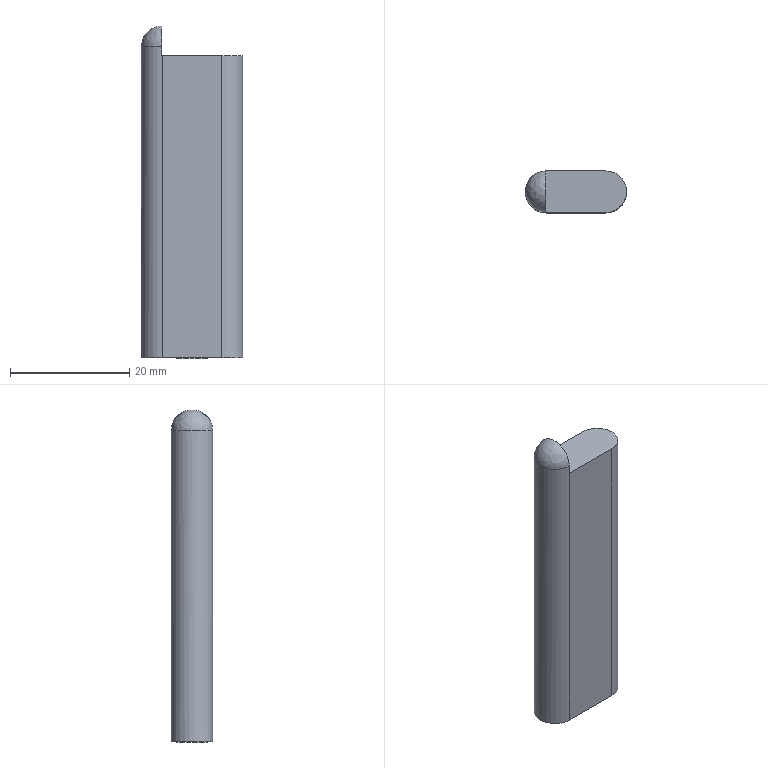Part | STEP file | LUOI GA TRON TREN | 1 solid | 15 faces | box 17 x 7 x 55.799 mm | volume 5306 mm3 | cylinder 5 | plane 5 | cone 4 | spline 1 | commonest cylinder face diameters 7 x3 4.134 x2
STEP:
#1=CARTESIAN_POINT('',(0.,0.,0.));
#2=DIRECTION('',(0.,0.,1.));
#3=DIRECTION('',(1.,0.,0.));
#4=AXIS2_PLACEMENT_3D('',#1,#2,#3);
#5=CARTESIAN_POINT('',(-3.5,0.,0.));
#6=VERTEX_POINT('',#5);
#7=CARTESIAN_POINT('',(0.,3.5,0.));
#8=VERTEX_POINT('',#7);
#9=CARTESIAN_POINT('',(-3.5,3.5,0.));
#10=DIRECTION('',(0.,0.,1.));
#11=DIRECTION('',(1.,0.,0.));
#12=AXIS2_PLACEMENT_3D('',#9,#10,#11);
#13=CIRCLE('',#12,3.5);
#14=CARTESIAN_POINT('',(-3.5,3.5,0.));
#15=DIRECTION('',(0.,0.,1.));
#16=DIRECTION('',(1.,0.,0.));
#17=AXIS2_PLACEMENT_3D('',#14,#15,#16);
#18=CYLINDRICAL_SURFACE('',#17,3.5);
#19=CARTESIAN_POINT('',(0.,0.));
#20=DIRECTION('',(1.,0.));
#21=VECTOR('',#20,1.);
#22=LINE('',#19,#21);
#23=(GEOMETRIC_REPRESENTATION_CONTEXT(2)PARAMETRIC_REPRESENTATION_CONTEXT()REPRESENTATION_CONTEXT('',''));
#24=DEFINITIONAL_REPRESENTATION('',(#22),#23);
#25=PCURVE('',#18,#24);
#26=CARTESIAN_POINT('',(-8.5,3.5,0.));
#27=DIRECTION('',(0.,0.,1.));
#28=DIRECTION('',(1.,0.,0.));
#29=AXIS2_PLACEMENT_3D('',#26,#27,#28);
#30=PLANE('',#29);
#31=CARTESIAN_POINT('',(5.,0.));
#32=DIRECTION('',(1.,0.));
#33=AXIS2_PLACEMENT_2D('',#31,#32);
#34=CIRCLE('',#33,3.5);
#35=(GEOMETRIC_REPRESENTATION_CONTEXT(2)PARAMETRIC_REPRESENTATION_CONTEXT()REPRESENTATION_CONTEXT('',''));
#36=DEFINITIONAL_REPRESENTATION('',(#34),#35);
#37=PCURVE('',#30,#36);
#38=SURFACE_CURVE('',#13,(#25,#37),.PCURVE_S1.);
#39=EDGE_CURVE('',#6,#8,#38,.T.);
#40=ORIENTED_EDGE('',*,*,#39,.T.);
#41=CARTESIAN_POINT('',(0.,3.5,50.8));
#42=VERTEX_POINT('',#41);
#43=CARTESIAN_POINT('',(0.,3.5,0.));
#44=DIRECTION('',(0.,0.,1.));
#45=VECTOR('',#44,1.);
#46=LINE('',#43,#45);
#47=CARTESIAN_POINT('',(6.283,0.));
#48=DIRECTION('',(0.,1.));
#49=VECTOR('',#48,1.);
#50=LINE('',#47,#49);
#51=(GEOMETRIC_REPRESENTATION_CONTEXT(2)PARAMETRIC_REPRESENTATION_CONTEXT()REPRESENTATION_CONTEXT('',''));
#52=DEFINITIONAL_REPRESENTATION('',(#50),#51);
#53=PCURVE('',#18,#52);
#54=CARTESIAN_POINT('',(-3.5,3.5,0.));
#55=DIRECTION('',(0.,0.,1.));
#56=DIRECTION('',(1.,0.,0.));
#57=AXIS2_PLACEMENT_3D('',#54,#55,#56);
#58=CYLINDRICAL_SURFACE('',#57,3.5);
#59=CARTESIAN_POINT('',(0.,0.));
#60=DIRECTION('',(0.,1.));
#61=VECTOR('',#60,1.);
#62=LINE('',#59,#61);
#63=(GEOMETRIC_REPRESENTATION_CONTEXT(2)PARAMETRIC_REPRESENTATION_CONTEXT()REPRESENTATION_CONTEXT('',''));
#64=DEFINITIONAL_REPRESENTATION('',(#62),#63);
#65=PCURVE('',#58,#64);
#66=SURFACE_CURVE('',#46,(#53,#65),.PCURVE_S1.);
#67=EDGE_CURVE('',#8,#42,#66,.T.);
#68=ORIENTED_EDGE('',*,*,#67,.T.);
#69=CARTESIAN_POINT('',(-3.5,0.,50.8));
#70=VERTEX_POINT('',#69);
#71=CARTESIAN_POINT('',(-3.5,3.5,50.8));
#72=DIRECTION('',(0.,0.,-1.));
#73=DIRECTION('',(1.,0.,0.));
#74=AXIS2_PLACEMENT_3D('',#71,#72,#73);
#75=CIRCLE('',#74,3.5);
#76=CARTESIAN_POINT('',(6.283,50.8));
#77=DIRECTION('',(-1.,0.));
#78=VECTOR('',#77,1.);
#79=LINE('',#76,#78);
#80=(GEOMETRIC_REPRESENTATION_CONTEXT(2)PARAMETRIC_REPRESENTATION_CONTEXT()REPRESENTATION_CONTEXT('',''));
#81=DEFINITIONAL_REPRESENTATION('',(#79),#80);
#82=PCURVE('',#18,#81);
#83=CARTESIAN_POINT('',(-13.6,0.,50.8));
#84=DIRECTION('',(0.,0.,-1.));
#85=DIRECTION('',(-1.,0.,0.));
#86=AXIS2_PLACEMENT_3D('',#83,#84,#85);
#87=PLANE('',#86);
#88=CARTESIAN_POINT('',(-10.1,3.5));
#89=DIRECTION('',(-1.,0.));
#90=AXIS2_PLACEMENT_2D('',#88,#89);
#91=CIRCLE('',#90,3.5);
#92=(GEOMETRIC_REPRESENTATION_CONTEXT(2)PARAMETRIC_REPRESENTATION_CONTEXT()REPRESENTATION_CONTEXT('',''));
#93=DEFINITIONAL_REPRESENTATION('',(#91),#92);
#94=PCURVE('',#87,#93);
#95=SURFACE_CURVE('',#75,(#82,#94),.PCURVE_S1.);
#96=EDGE_CURVE('',#42,#70,#95,.T.);
#97=ORIENTED_EDGE('',*,*,#96,.T.);
#98=CARTESIAN_POINT('',(-3.5,0.,0.));
#99=DIRECTION('',(0.,0.,1.));
#100=VECTOR('',#99,1.);
#101=LINE('',#98,#100);
#102=CARTESIAN_POINT('',(4.712,0.));
#103=DIRECTION('',(0.,1.));
#104=VECTOR('',#103,1.);
#105=LINE('',#102,#104);
#106=(GEOMETRIC_REPRESENTATION_CONTEXT(2)PARAMETRIC_REPRESENTATION_CONTEXT()REPRESENTATION_CONTEXT('',''));
#107=DEFINITIONAL_REPRESENTATION('',(#105),#106);
#108=PCURVE('',#18,#107);
#109=CARTESIAN_POINT('',(0.,0.,0.));
#110=DIRECTION('',(0.,-1.,0.));
#111=DIRECTION('',(0.,0.,-1.));
#112=AXIS2_PLACEMENT_3D('',#109,#110,#111);
#113=PLANE('',#112);
#114=CARTESIAN_POINT('',(0.,-3.5));
#115=DIRECTION('',(-1.,0.));
#116=VECTOR('',#115,1.);
#117=LINE('',#114,#116);
#118=(GEOMETRIC_REPRESENTATION_CONTEXT(2)PARAMETRIC_REPRESENTATION_CONTEXT()REPRESENTATION_CONTEXT('',''));
#119=DEFINITIONAL_REPRESENTATION('',(#117),#118);
#120=PCURVE('',#113,#119);
#121=SURFACE_CURVE('',#101,(#108,#120),.PCURVE_S1.);
#122=EDGE_CURVE('',#6,#70,#121,.T.);
#123=ORIENTED_EDGE('',*,*,#122,.F.);
#124=EDGE_LOOP('',(#40,#68,#97,#123));
#125=FACE_BOUND('',#124,.T.);
#126=ADVANCED_FACE('',(#125),#18,.T.);
#127=CARTESIAN_POINT('',(-10.567,3.5,0.5));
#128=VERTEX_POINT('',#127);
#129=CARTESIAN_POINT('',(-11.067,3.5,0.));
#130=VERTEX_POINT('',#129);
#131=CARTESIAN_POINT('',(-11.067,3.5,0.));
#132=DIRECTION('',(-0.7071,0.,-0.7071));
#133=VECTOR('',#132,1.);
#134=LINE('',#131,#133);
#135=CARTESIAN_POINT('',(-8.5,3.5,0.));
#136=DIRECTION('',(0.,0.,-1.));
#137=DIRECTION('',(-1.,0.,0.));
#138=AXIS2_PLACEMENT_3D('',#135,#136,#137);
#139=CONICAL_SURFACE('',#138,2.567,0.7854);
#140=CARTESIAN_POINT('',(6.283,0.));
#141=DIRECTION('',(0.,1.));
#142=VECTOR('',#141,1.);
#143=LINE('',#140,#142);
#144=(GEOMETRIC_REPRESENTATION_CONTEXT(2)PARAMETRIC_REPRESENTATION_CONTEXT()REPRESENTATION_CONTEXT('',''));
#145=DEFINITIONAL_REPRESENTATION('',(#143),#144);
#146=PCURVE('',#139,#145);
#147=CARTESIAN_POINT('',(-8.5,3.5,0.));
#148=DIRECTION('',(0.,0.,-1.));
#149=DIRECTION('',(-1.,0.,0.));
#150=AXIS2_PLACEMENT_3D('',#147,#148,#149);
#151=CONICAL_SURFACE('',#150,2.567,0.7854);
#152=CARTESIAN_POINT('',(0.,0.));
#153=DIRECTION('',(0.,1.));
#154=VECTOR('',#153,1.);
#155=LINE('',#152,#154);
#156=(GEOMETRIC_REPRESENTATION_CONTEXT(2)PARAMETRIC_REPRESENTATION_CONTEXT()REPRESENTATION_CONTEXT('',''));
#157=DEFINITIONAL_REPRESENTATION('',(#155),#156);
#158=PCURVE('',#151,#157);
#159=SURFACE_CURVE('',#134,(#146,#158),.PCURVE_S1.);
#160=EDGE_CURVE('',#128,#130,#159,.T.);
#161=ORIENTED_EDGE('',*,*,#160,.T.);
#162=CARTESIAN_POINT('',(-5.933,3.5,0.));
#163=VERTEX_POINT('',#162);
#164=CARTESIAN_POINT('',(-8.5,3.5,0.));
#165=DIRECTION('',(0.,0.,-1.));
#166=DIRECTION('',(-1.,0.,0.));
#167=AXIS2_PLACEMENT_3D('',#164,#165,#166);
#168=CIRCLE('',#167,2.567);
#169=CARTESIAN_POINT('',(0.,0.));
#170=DIRECTION('',(1.,0.));
#171=VECTOR('',#170,1.);
#172=LINE('',#169,#171);
#173=(GEOMETRIC_REPRESENTATION_CONTEXT(2)PARAMETRIC_REPRESENTATION_CONTEXT()REPRESENTATION_CONTEXT('',''));
#174=DEFINITIONAL_REPRESENTATION('',(#172),#173);
#175=PCURVE('',#139,#174);
#176=CARTESIAN_POINT('',(-2.567,0.));
#177=CARTESIAN_POINT('',(-2.567,4.446));
#178=CARTESIAN_POINT('',(1.283,2.223));
#179=CARTESIAN_POINT('',(5.134,0.));
#180=CARTESIAN_POINT('',(1.283,-2.223));
#181=CARTESIAN_POINT('',(-2.567,-4.446));
#182=CARTESIAN_POINT('',(-2.567,0.));
#183=(BOUNDED_CURVE()B_SPLINE_CURVE(2,(#176,#177,#178,#179,#180,#181,#182),.UNSPECIFIED.,.T.,.F.)B_SPLINE_CURVE_WITH_KNOTS((1,2,2,2,2,1),(-2.094,0.,2.094,4.189,6.283,8.378),.UNSPECIFIED.)CURVE()GEOMETRIC_REPRESENTATION_ITEM()RATIONAL_B_SPLINE_CURVE((1.,0.5,1.,0.5,1.,0.5,1.))REPRESENTATION_ITEM(''));
#184=(GEOMETRIC_REPRESENTATION_CONTEXT(2)PARAMETRIC_REPRESENTATION_CONTEXT()REPRESENTATION_CONTEXT('',''));
#185=DEFINITIONAL_REPRESENTATION('',(#183),#184);
#186=PCURVE('',#30,#185);
#187=SURFACE_CURVE('',#168,(#175,#186),.PCURVE_S1.);
#188=EDGE_CURVE('',#163,#130,#187,.T.);
#189=ORIENTED_EDGE('',*,*,#188,.F.);
#190=CARTESIAN_POINT('',(-6.433,3.5,0.5));
#191=VERTEX_POINT('',#190);
#192=CARTESIAN_POINT('',(-5.933,3.5,0.));
#193=DIRECTION('',(0.7071,0.,-0.7071));
#194=VECTOR('',#193,1.);
#195=LINE('',#192,#194);
#196=CARTESIAN_POINT('',(3.142,0.));
#197=DIRECTION('',(0.,1.));
#198=VECTOR('',#197,1.);
#199=LINE('',#196,#198);
#200=(GEOMETRIC_REPRESENTATION_CONTEXT(2)PARAMETRIC_REPRESENTATION_CONTEXT()REPRESENTATION_CONTEXT('',''));
#201=DEFINITIONAL_REPRESENTATION('',(#199),#200);
#202=PCURVE('',#139,#201);
#203=CARTESIAN_POINT('',(3.142,0.));
#204=DIRECTION('',(0.,1.));
#205=VECTOR('',#204,1.);
#206=LINE('',#203,#205);
#207=(GEOMETRIC_REPRESENTATION_CONTEXT(2)PARAMETRIC_REPRESENTATION_CONTEXT()REPRESENTATION_CONTEXT('',''));
#208=DEFINITIONAL_REPRESENTATION('',(#206),#207);
#209=PCURVE('',#151,#208);
#210=SURFACE_CURVE('',#195,(#202,#209),.PCURVE_S1.);
#211=EDGE_CURVE('',#191,#163,#210,.T.);
#212=ORIENTED_EDGE('',*,*,#211,.F.);
#213=CARTESIAN_POINT('',(-8.5,3.5,0.5));
#214=DIRECTION('',(0.,0.,-1.));
#215=DIRECTION('',(1.,0.,0.));
#216=AXIS2_PLACEMENT_3D('',#213,#214,#215);
#217=CIRCLE('',#216,2.067);
#218=CARTESIAN_POINT('',(3.142,-0.5));
#219=DIRECTION('',(1.,0.));
#220=VECTOR('',#219,1.);
#221=LINE('',#218,#220);
#222=(GEOMETRIC_REPRESENTATION_CONTEXT(2)PARAMETRIC_REPRESENTATION_CONTEXT()REPRESENTATION_CONTEXT('',''));
#223=DEFINITIONAL_REPRESENTATION('',(#221),#222);
#224=PCURVE('',#139,#223);
#225=CARTESIAN_POINT('',(-8.5,3.5,10.));
#226=DIRECTION('',(0.,0.,-1.));
#227=DIRECTION('',(-1.,0.,0.));
#228=AXIS2_PLACEMENT_3D('',#225,#226,#227);
#229=CYLINDRICAL_SURFACE('',#228,2.067);
#230=CARTESIAN_POINT('',(3.142,9.5));
#231=DIRECTION('',(1.,0.));
#232=VECTOR('',#231,1.);
#233=LINE('',#230,#232);
#234=(GEOMETRIC_REPRESENTATION_CONTEXT(2)PARAMETRIC_REPRESENTATION_CONTEXT()REPRESENTATION_CONTEXT('',''));
#235=DEFINITIONAL_REPRESENTATION('',(#233),#234);
#236=PCURVE('',#229,#235);
#237=SURFACE_CURVE('',#217,(#224,#236),.PCURVE_S1.);
#238=EDGE_CURVE('',#191,#128,#237,.T.);
#239=ORIENTED_EDGE('',*,*,#238,.T.);
#240=EDGE_LOOP('',(#161,#189,#212,#239));
#241=FACE_BOUND('',#240,.F.);
#242=ADVANCED_FACE('',(#241),#139,.F.);
#243=CARTESIAN_POINT('',(-10.567,3.5,20.));
#244=VERTEX_POINT('',#243);
#245=CARTESIAN_POINT('',(-10.567,3.5,10.));
#246=DIRECTION('',(0.,0.,-1.));
#247=VECTOR('',#246,1.);
#248=LINE('',#245,#247);
#249=CARTESIAN_POINT('',(6.283,0.));
#250=DIRECTION('',(0.,1.));
#251=VECTOR('',#250,1.);
#252=LINE('',#249,#251);
#253=(GEOMETRIC_REPRESENTATION_CONTEXT(2)PARAMETRIC_REPRESENTATION_CONTEXT()REPRESENTATION_CONTEXT('',''));
#254=DEFINITIONAL_REPRESENTATION('',(#252),#253);
#255=PCURVE('',#229,#254);
#256=CARTESIAN_POINT('',(-8.5,3.5,10.));
#257=DIRECTION('',(0.,0.,-1.));
#258=DIRECTION('',(-1.,0.,0.));
#259=AXIS2_PLACEMENT_3D('',#256,#257,#258);
#260=CYLINDRICAL_SURFACE('',#259,2.067);
#261=CARTESIAN_POINT('',(0.,0.));
#262=DIRECTION('',(0.,1.));
#263=VECTOR('',#262,1.);
#264=LINE('',#261,#263);
#265=(GEOMETRIC_REPRESENTATION_CONTEXT(2)PARAMETRIC_REPRESENTATION_CONTEXT()REPRESENTATION_CONTEXT('',''));
#266=DEFINITIONAL_REPRESENTATION('',(#264),#265);
#267=PCURVE('',#260,#266);
#268=SURFACE_CURVE('',#248,(#255,#267),.PCURVE_S1.);
#269=EDGE_CURVE('',#244,#128,#268,.T.);
#270=ORIENTED_EDGE('',*,*,#269,.T.);
#271=ORIENTED_EDGE('',*,*,#238,.F.);
#272=CARTESIAN_POINT('',(-6.433,3.5,20.));
#273=VERTEX_POINT('',#272);
#274=CARTESIAN_POINT('',(-6.433,3.5,10.));
#275=DIRECTION('',(0.,0.,-1.));
#276=VECTOR('',#275,1.);
#277=LINE('',#274,#276);
#278=CARTESIAN_POINT('',(3.142,0.));
#279=DIRECTION('',(0.,1.));
#280=VECTOR('',#279,1.);
#281=LINE('',#278,#280);
#282=(GEOMETRIC_REPRESENTATION_CONTEXT(2)PARAMETRIC_REPRESENTATION_CONTEXT()REPRESENTATION_CONTEXT('',''));
#283=DEFINITIONAL_REPRESENTATION('',(#281),#282);
#284=PCURVE('',#229,#283);
#285=CARTESIAN_POINT('',(3.142,0.));
#286=DIRECTION('',(0.,1.));
#287=VECTOR('',#286,1.);
#288=LINE('',#285,#287);
#289=(GEOMETRIC_REPRESENTATION_CONTEXT(2)PARAMETRIC_REPRESENTATION_CONTEXT()REPRESENTATION_CONTEXT('',''));
#290=DEFINITIONAL_REPRESENTATION('',(#288),#289);
#291=PCURVE('',#260,#290);
#292=SURFACE_CURVE('',#277,(#284,#291),.PCURVE_S1.);
#293=EDGE_CURVE('',#273,#191,#292,.T.);
#294=ORIENTED_EDGE('',*,*,#293,.F.);
#295=CARTESIAN_POINT('',(-8.5,3.5,20.));
#296=DIRECTION('',(0.,0.,-1.));
#297=DIRECTION('',(-1.,0.,0.));
#298=AXIS2_PLACEMENT_3D('',#295,#296,#297);
#299=CIRCLE('',#298,2.067);
#300=CARTESIAN_POINT('',(0.,-10.));
#301=DIRECTION('',(1.,0.));
#302=VECTOR('',#301,1.);
#303=LINE('',#300,#302);
#304=(GEOMETRIC_REPRESENTATION_CONTEXT(2)PARAMETRIC_REPRESENTATION_CONTEXT()REPRESENTATION_CONTEXT('',''));
#305=DEFINITIONAL_REPRESENTATION('',(#303),#304);
#306=PCURVE('',#229,#305);
#307=CARTESIAN_POINT('',(-8.5,3.5,20.));
#308=DIRECTION('',(0.,0.,-1.));
#309=DIRECTION('',(-1.,0.,0.));
#310=AXIS2_PLACEMENT_3D('',#307,#308,#309);
#311=CONICAL_SURFACE('',#310,2.067,1.03);
#312=CARTESIAN_POINT('',(0.,0.));
#313=DIRECTION('',(1.,0.));
#314=VECTOR('',#313,1.);
#315=LINE('',#312,#314);
#316=(GEOMETRIC_REPRESENTATION_CONTEXT(2)PARAMETRIC_REPRESENTATION_CONTEXT()REPRESENTATION_CONTEXT('',''));
#317=DEFINITIONAL_REPRESENTATION('',(#315),#316);
#318=PCURVE('',#311,#317);
#319=SURFACE_CURVE('',#299,(#306,#318),.PCURVE_S1.);
#320=EDGE_CURVE('',#273,#244,#319,.T.);
#321=ORIENTED_EDGE('',*,*,#320,.T.);
#322=EDGE_LOOP('',(#270,#271,#294,#321));
#323=FACE_BOUND('',#322,.F.);
#324=ADVANCED_FACE('',(#323),#229,.F.);
#325=ORIENTED_EDGE('',*,*,#320,.F.);
#326=CARTESIAN_POINT('',(-8.5,3.5,21.242));
#327=VERTEX_POINT('',#326);
#328=CARTESIAN_POINT('',(-6.433,3.5,20.));
#329=DIRECTION('',(0.8572,0.,-0.515));
#330=VECTOR('',#329,1.);
#331=LINE('',#328,#330);
#332=CARTESIAN_POINT('',(3.142,0.));
#333=DIRECTION('',(0.,1.));
#334=VECTOR('',#333,1.);
#335=LINE('',#332,#334);
#336=(GEOMETRIC_REPRESENTATION_CONTEXT(2)PARAMETRIC_REPRESENTATION_CONTEXT()REPRESENTATION_CONTEXT('',''));
#337=DEFINITIONAL_REPRESENTATION('',(#335),#336);
#338=PCURVE('',#311,#337);
#339=CARTESIAN_POINT('',(-8.5,3.5,20.));
#340=DIRECTION('',(0.,0.,-1.));
#341=DIRECTION('',(-1.,0.,0.));
#342=AXIS2_PLACEMENT_3D('',#339,#340,#341);
#343=CONICAL_SURFACE('',#342,2.067,1.03);
#344=CARTESIAN_POINT('',(3.142,0.));
#345=DIRECTION('',(0.,1.));
#346=VECTOR('',#345,1.);
#347=LINE('',#344,#346);
#348=(GEOMETRIC_REPRESENTATION_CONTEXT(2)PARAMETRIC_REPRESENTATION_CONTEXT()REPRESENTATION_CONTEXT('',''));
#349=DEFINITIONAL_REPRESENTATION('',(#347),#348);
#350=PCURVE('',#343,#349);
#351=SURFACE_CURVE('',#331,(#338,#350),.PCURVE_S1.);
#352=EDGE_CURVE('',#327,#273,#351,.T.);
#353=ORIENTED_EDGE('',*,*,#352,.F.);
#354=CARTESIAN_POINT('',(-10.567,3.5,20.));
#355=DIRECTION('',(-0.8572,0.,-0.515));
#356=VECTOR('',#355,1.);
#357=LINE('',#354,#356);
#358=CARTESIAN_POINT('',(6.283,0.));
#359=DIRECTION('',(0.,1.));
#360=VECTOR('',#359,1.);
#361=LINE('',#358,#360);
#362=(GEOMETRIC_REPRESENTATION_CONTEXT(2)PARAMETRIC_REPRESENTATION_CONTEXT()REPRESENTATION_CONTEXT('',''));
#363=DEFINITIONAL_REPRESENTATION('',(#361),#362);
#364=PCURVE('',#311,#363);
#365=CARTESIAN_POINT('',(0.,0.));
#366=DIRECTION('',(0.,1.));
#367=VECTOR('',#366,1.);
#368=LINE('',#365,#367);
#369=(GEOMETRIC_REPRESENTATION_CONTEXT(2)PARAMETRIC_REPRESENTATION_CONTEXT()REPRESENTATION_CONTEXT('',''));
#370=DEFINITIONAL_REPRESENTATION('',(#368),#369);
#371=PCURVE('',#343,#370);
#372=SURFACE_CURVE('',#357,(#364,#371),.PCURVE_S1.);
#373=EDGE_CURVE('',#327,#244,#372,.T.);
#374=ORIENTED_EDGE('',*,*,#373,.T.);
#375=EDGE_LOOP('',(#325,#353,#374));
#376=FACE_BOUND('',#375,.F.);
#377=ADVANCED_FACE('',(#376),#311,.F.);
#378=CARTESIAN_POINT('',(-13.5,0.,50.8));
#379=VERTEX_POINT('',#378);
#380=CARTESIAN_POINT('',(-13.6,0.001429,50.8));
#381=VERTEX_POINT('',#380);
#382=CARTESIAN_POINT('',(-13.5,3.5,50.8));
#383=DIRECTION('',(0.,0.,-1.));
#384=DIRECTION('',(1.,0.,0.));
#385=AXIS2_PLACEMENT_3D('',#382,#383,#384);
#386=CIRCLE('',#385,3.5);
#387=CARTESIAN_POINT('',(-13.5,3.5,0.));
#388=DIRECTION('',(0.,0.,1.));
#389=DIRECTION('',(1.,0.,0.));
#390=AXIS2_PLACEMENT_3D('',#387,#388,#389);
#391=CYLINDRICAL_SURFACE('',#390,3.5);
#392=CARTESIAN_POINT('',(6.283,50.8));
#393=DIRECTION('',(-1.,0.));
#394=VECTOR('',#393,1.);
#395=LINE('',#392,#394);
#396=(GEOMETRIC_REPRESENTATION_CONTEXT(2)PARAMETRIC_REPRESENTATION_CONTEXT()REPRESENTATION_CONTEXT('',''));
#397=DEFINITIONAL_REPRESENTATION('',(#395),#396);
#398=PCURVE('',#391,#397);
#399=CARTESIAN_POINT('',(-0.1,3.5));
#400=DIRECTION('',(-1.,0.));
#401=AXIS2_PLACEMENT_2D('',#399,#400);
#402=CIRCLE('',#401,3.5);
#403=(GEOMETRIC_REPRESENTATION_CONTEXT(2)PARAMETRIC_REPRESENTATION_CONTEXT()REPRESENTATION_CONTEXT('',''));
#404=DEFINITIONAL_REPRESENTATION('',(#402),#403);
#405=PCURVE('',#87,#404);
#406=SURFACE_CURVE('',#386,(#398,#405),.PCURVE_S1.);
#407=EDGE_CURVE('',#379,#381,#406,.T.);
#408=ORIENTED_EDGE('',*,*,#407,.T.);
#409=CARTESIAN_POINT('',(-13.6,0.001429,52.3));
#410=VERTEX_POINT('',#409);
#411=CARTESIAN_POINT('',(-13.6,0.001429,57.857));
#412=DIRECTION('',(0.,0.,1.));
#413=VECTOR('',#412,1.);
#414=LINE('',#411,#413);
#415=CARTESIAN_POINT('',(4.684,57.857));
#416=DIRECTION('',(0.,1.));
#417=VECTOR('',#416,1.);
#418=LINE('',#415,#417);
#419=(GEOMETRIC_REPRESENTATION_CONTEXT(2)PARAMETRIC_REPRESENTATION_CONTEXT()REPRESENTATION_CONTEXT('',''));
#420=DEFINITIONAL_REPRESENTATION('',(#418),#419);
#421=PCURVE('',#391,#420);
#422=CARTESIAN_POINT('',(-13.6,0.,57.857));
#423=DIRECTION('',(-1.,0.,0.));
#424=DIRECTION('',(0.,0.,1.));
#425=AXIS2_PLACEMENT_3D('',#422,#423,#424);
#426=PLANE('',#425);
#427=CARTESIAN_POINT('',(0.,0.001429));
#428=DIRECTION('',(1.,0.));
#429=VECTOR('',#428,1.);
#430=LINE('',#427,#429);
#431=(GEOMETRIC_REPRESENTATION_CONTEXT(2)PARAMETRIC_REPRESENTATION_CONTEXT()REPRESENTATION_CONTEXT('',''));
#432=DEFINITIONAL_REPRESENTATION('',(#430),#431);
#433=PCURVE('',#426,#432);
#434=SURFACE_CURVE('',#414,(#421,#433),.PCURVE_S1.);
#435=EDGE_CURVE('',#381,#410,#434,.T.);
#436=ORIENTED_EDGE('',*,*,#435,.T.);
#437=CARTESIAN_POINT('',(-17.,3.5,52.3));
#438=VERTEX_POINT('',#437);
#439=CARTESIAN_POINT('',(-13.5,3.5,52.3));
#440=DIRECTION('',(0.,0.,-1.));
#441=DIRECTION('',(1.,0.,0.));
#442=AXIS2_PLACEMENT_3D('',#439,#440,#441);
#443=CIRCLE('',#442,3.5);
#444=CARTESIAN_POINT('',(6.283,52.3));
#445=DIRECTION('',(-1.,0.));
#446=VECTOR('',#445,1.);
#447=LINE('',#444,#446);
#448=(GEOMETRIC_REPRESENTATION_CONTEXT(2)PARAMETRIC_REPRESENTATION_CONTEXT()REPRESENTATION_CONTEXT('',''));
#449=DEFINITIONAL_REPRESENTATION('',(#447),#448);
#450=PCURVE('',#391,#449);
#451=CARTESIAN_POINT('',(-13.6,6.999,52.3));
#452=CARTESIAN_POINT('',(-13.6,6.999,59.297));
#453=CARTESIAN_POINT('',(-13.6,0.001429,59.297));
#454=CARTESIAN_POINT('',(-13.6,0.001429,52.3));
#455=CARTESIAN_POINT('',(-15.603,6.941,52.3));
#456=CARTESIAN_POINT('',(-15.603,6.941,59.183));
#457=CARTESIAN_POINT('',(-15.603,0.05869,59.183));
#458=CARTESIAN_POINT('',(-15.603,0.05869,52.3));
#459=CARTESIAN_POINT('',(-17.,5.504,52.3));
#460=CARTESIAN_POINT('',(-17.,5.504,56.308));
#461=CARTESIAN_POINT('',(-17.,1.496,56.308));
#462=CARTESIAN_POINT('',(-17.,1.496,52.3));
#463=CARTESIAN_POINT('',(-17.,3.5,52.3));
#464=CARTESIAN_POINT('',(-17.,3.5,52.3));
#465=CARTESIAN_POINT('',(-17.,3.5,52.3));
#466=CARTESIAN_POINT('',(-17.,3.5,52.3));
#467=(BOUNDED_SURFACE()B_SPLINE_SURFACE(3,3,((#451,#452,#453,#454),(#455,#456,#457,#458),(#459,#460,#461,#462),(#463,#464,#465,#466)),.UNSPECIFIED.,.F.,.F.,.F.)B_SPLINE_SURFACE_WITH_KNOTS((4,4),(4,4),(0.,1.),(0.,1.),.PIECEWISE_BEZIER_KNOTS.)GEOMETRIC_REPRESENTATION_ITEM()RATIONAL_B_SPLINE_SURFACE(((1.,0.3333,0.3333,1.),(0.8114,0.2705,0.2705,0.8114),(0.8114,0.2705,0.2705,0.8114),(1.,0.3333,0.3333,1.)))REPRESENTATION_ITEM('')SURFACE());
#468=CARTESIAN_POINT('',(0.,1.));
#469=CARTESIAN_POINT('',(0.01676,1.));
#470=CARTESIAN_POINT('',(0.04982,1.));
#471=CARTESIAN_POINT('',(0.09814,1.));
#472=CARTESIAN_POINT('',(0.1454,1.));
#473=CARTESIAN_POINT('',(0.1917,1.));
#474=CARTESIAN_POINT('',(0.2371,1.));
#475=CARTESIAN_POINT('',(0.282,1.));
#476=CARTESIAN_POINT('',(0.3262,1.));
#477=CARTESIAN_POINT('',(0.37,1.));
#478=CARTESIAN_POINT('',(0.4135,1.));
#479=CARTESIAN_POINT('',(0.4568,1.));
#480=CARTESIAN_POINT('',(0.5,1.));
#481=CARTESIAN_POINT('',(0.5432,1.));
#482=CARTESIAN_POINT('',(0.5865,1.));
#483=CARTESIAN_POINT('',(0.63,1.));
#484=CARTESIAN_POINT('',(0.6738,1.));
#485=CARTESIAN_POINT('',(0.718,1.));
#486=CARTESIAN_POINT('',(0.7629,1.));
#487=CARTESIAN_POINT('',(0.8083,1.));
#488=CARTESIAN_POINT('',(0.8546,1.));
#489=CARTESIAN_POINT('',(0.9019,1.));
#490=CARTESIAN_POINT('',(0.9502,1.));
#491=CARTESIAN_POINT('',(0.9832,1.));
#492=CARTESIAN_POINT('',(1.,1.));
#493=B_SPLINE_CURVE_WITH_KNOTS('',3,(#468,#469,#470,#471,#472,#473,#474,#475,#476,#477,#478,#479,#480,#481,#482,#483,#484,#485,#486,#487,#488,#489,#490,#491,#492),.UNSPECIFIED.,.F.,.F.,(4,1,1,1,1,1,1,1,1,1,1,1,1,1,1,1,1,1,1,1,1,1,4),(1.599,1.669,1.74,1.81,1.88,1.95,2.02,2.09,2.16,2.23,2.3,2.37,2.441,2.511,2.581,2.651,2.721,2.791,2.861,2.931,3.001,3.071,3.142),.QUASI_UNIFORM_KNOTS.);
#494=(GEOMETRIC_REPRESENTATION_CONTEXT(2)PARAMETRIC_REPRESENTATION_CONTEXT()REPRESENTATION_CONTEXT('',''));
#495=DEFINITIONAL_REPRESENTATION('',(#493),#494);
#496=PCURVE('',#467,#495);
#497=SURFACE_CURVE('',#443,(#450,#496),.PCURVE_S1.);
#498=EDGE_CURVE('',#410,#438,#497,.T.);
#499=ORIENTED_EDGE('',*,*,#498,.T.);
#500=CARTESIAN_POINT('',(-13.6,6.999,52.3));
#501=VERTEX_POINT('',#500);
#502=CARTESIAN_POINT('',(-13.5,3.5,52.3));
#503=DIRECTION('',(0.,0.,-1.));
#504=DIRECTION('',(1.,0.,0.));
#505=AXIS2_PLACEMENT_3D('',#502,#503,#504);
#506=CIRCLE('',#505,3.5);
#507=CARTESIAN_POINT('',(6.283,52.3));
#508=DIRECTION('',(-1.,0.));
#509=VECTOR('',#508,1.);
#510=LINE('',#507,#509);
#511=(GEOMETRIC_REPRESENTATION_CONTEXT(2)PARAMETRIC_REPRESENTATION_CONTEXT()REPRESENTATION_CONTEXT('',''));
#512=DEFINITIONAL_REPRESENTATION('',(#510),#511);
#513=PCURVE('',#391,#512);
#514=CARTESIAN_POINT('',(1.,0.));
#515=CARTESIAN_POINT('',(0.9832,0.));
#516=CARTESIAN_POINT('',(0.9502,0.));
#517=CARTESIAN_POINT('',(0.9019,0.));
#518=CARTESIAN_POINT('',(0.8546,0.));
#519=CARTESIAN_POINT('',(0.8083,0.));
#520=CARTESIAN_POINT('',(0.7629,0.));
#521=CARTESIAN_POINT('',(0.718,0.));
#522=CARTESIAN_POINT('',(0.6738,0.));
#523=CARTESIAN_POINT('',(0.63,0.));
#524=CARTESIAN_POINT('',(0.5865,0.));
#525=CARTESIAN_POINT('',(0.5432,0.));
#526=CARTESIAN_POINT('',(0.5,0.));
#527=CARTESIAN_POINT('',(0.4568,0.));
#528=CARTESIAN_POINT('',(0.4135,0.));
#529=CARTESIAN_POINT('',(0.37,0.));
#530=CARTESIAN_POINT('',(0.3262,0.));
#531=CARTESIAN_POINT('',(0.282,0.));
#532=CARTESIAN_POINT('',(0.2371,0.));
#533=CARTESIAN_POINT('',(0.1917,0.));
#534=CARTESIAN_POINT('',(0.1454,0.));
#535=CARTESIAN_POINT('',(0.09814,0.));
#536=CARTESIAN_POINT('',(0.04982,0.));
#537=CARTESIAN_POINT('',(0.01676,0.));
#538=CARTESIAN_POINT('',(0.,0.));
#539=B_SPLINE_CURVE_WITH_KNOTS('',3,(#514,#515,#516,#517,#518,#519,#520,#521,#522,#523,#524,#525,#526,#527,#528,#529,#530,#531,#532,#533,#534,#535,#536,#537,#538),.UNSPECIFIED.,.F.,.F.,(4,1,1,1,1,1,1,1,1,1,1,1,1,1,1,1,1,1,1,1,1,1,4),(3.142,3.212,3.282,3.352,3.422,3.492,3.562,3.632,3.702,3.773,3.843,3.913,3.983,4.053,4.123,4.193,4.263,4.333,4.403,4.474,4.544,4.614,4.684),.QUASI_UNIFORM_KNOTS.);
#540=(GEOMETRIC_REPRESENTATION_CONTEXT(2)PARAMETRIC_REPRESENTATION_CONTEXT()REPRESENTATION_CONTEXT('',''));
#541=DEFINITIONAL_REPRESENTATION('',(#539),#540);
#542=PCURVE('',#467,#541);
#543=SURFACE_CURVE('',#506,(#513,#542),.PCURVE_S1.);
#544=EDGE_CURVE('',#438,#501,#543,.T.);
#545=ORIENTED_EDGE('',*,*,#544,.T.);
#546=CARTESIAN_POINT('',(-13.6,6.999,50.8));
#547=VERTEX_POINT('',#546);
#548=CARTESIAN_POINT('',(-13.6,6.999,57.857));
#549=DIRECTION('',(0.,0.,-1.));
#550=VECTOR('',#549,1.);
#551=LINE('',#548,#550);
#552=CARTESIAN_POINT('',(1.599,57.857));
#553=DIRECTION('',(0.,-1.));
#554=VECTOR('',#553,1.);
#555=LINE('',#552,#554);
#556=(GEOMETRIC_REPRESENTATION_CONTEXT(2)PARAMETRIC_REPRESENTATION_CONTEXT()REPRESENTATION_CONTEXT('',''));
#557=DEFINITIONAL_REPRESENTATION('',(#555),#556);
#558=PCURVE('',#391,#557);
#559=CARTESIAN_POINT('',(0.,6.999));
#560=DIRECTION('',(-1.,0.));
#561=VECTOR('',#560,1.);
#562=LINE('',#559,#561);
#563=(GEOMETRIC_REPRESENTATION_CONTEXT(2)PARAMETRIC_REPRESENTATION_CONTEXT()REPRESENTATION_CONTEXT('',''));
#564=DEFINITIONAL_REPRESENTATION('',(#562),#563);
#565=PCURVE('',#426,#564);
#566=SURFACE_CURVE('',#551,(#558,#565),.PCURVE_S1.);
#567=EDGE_CURVE('',#501,#547,#566,.T.);
#568=ORIENTED_EDGE('',*,*,#567,.T.);
#569=CARTESIAN_POINT('',(-13.5,7.,50.8));
#570=VERTEX_POINT('',#569);
#571=CARTESIAN_POINT('',(-13.5,3.5,50.8));
#572=DIRECTION('',(0.,0.,-1.));
#573=DIRECTION('',(1.,0.,0.));
#574=AXIS2_PLACEMENT_3D('',#571,#572,#573);
#575=CIRCLE('',#574,3.5);
#576=CARTESIAN_POINT('',(6.283,50.8));
#577=DIRECTION('',(-1.,0.));
#578=VECTOR('',#577,1.);
#579=LINE('',#576,#578);
#580=(GEOMETRIC_REPRESENTATION_CONTEXT(2)PARAMETRIC_REPRESENTATION_CONTEXT()REPRESENTATION_CONTEXT('',''));
#581=DEFINITIONAL_REPRESENTATION('',(#579),#580);
#582=PCURVE('',#391,#581);
#583=CARTESIAN_POINT('',(-0.1,3.5));
#584=DIRECTION('',(-1.,0.));
#585=AXIS2_PLACEMENT_2D('',#583,#584);
#586=CIRCLE('',#585,3.5);
#587=(GEOMETRIC_REPRESENTATION_CONTEXT(2)PARAMETRIC_REPRESENTATION_CONTEXT()REPRESENTATION_CONTEXT('',''));
#588=DEFINITIONAL_REPRESENTATION('',(#586),#587);
#589=PCURVE('',#87,#588);
#590=SURFACE_CURVE('',#575,(#582,#589),.PCURVE_S1.);
#591=EDGE_CURVE('',#547,#570,#590,.T.);
#592=ORIENTED_EDGE('',*,*,#591,.T.);
#593=CARTESIAN_POINT('',(-13.5,7.,0.));
#594=VERTEX_POINT('',#593);
#595=CARTESIAN_POINT('',(-13.5,7.,0.));
#596=DIRECTION('',(0.,0.,-1.));
#597=VECTOR('',#596,1.);
#598=LINE('',#595,#597);
#599=CARTESIAN_POINT('',(1.571,0.));
#600=DIRECTION('',(0.,-1.));
#601=VECTOR('',#600,1.);
#602=LINE('',#599,#601);
#603=(GEOMETRIC_REPRESENTATION_CONTEXT(2)PARAMETRIC_REPRESENTATION_CONTEXT()REPRESENTATION_CONTEXT('',''));
#604=DEFINITIONAL_REPRESENTATION('',(#602),#603);
#605=PCURVE('',#391,#604);
#606=CARTESIAN_POINT('',(-17.,7.,0.));
#607=DIRECTION('',(0.,1.,0.));
#608=DIRECTION('',(0.,0.,1.));
#609=AXIS2_PLACEMENT_3D('',#606,#607,#608);
#610=PLANE('',#609);
#611=CARTESIAN_POINT('',(0.,3.5));
#612=DIRECTION('',(-1.,0.));
#613=VECTOR('',#612,1.);
#614=LINE('',#611,#613);
#615=(GEOMETRIC_REPRESENTATION_CONTEXT(2)PARAMETRIC_REPRESENTATION_CONTEXT()REPRESENTATION_CONTEXT('',''));
#616=DEFINITIONAL_REPRESENTATION('',(#614),#615);
#617=PCURVE('',#610,#616);
#618=SURFACE_CURVE('',#598,(#605,#617),.PCURVE_S1.);
#619=EDGE_CURVE('',#570,#594,#618,.T.);
#620=ORIENTED_EDGE('',*,*,#619,.T.);
#621=CARTESIAN_POINT('',(-13.5,0.,0.));
#622=VERTEX_POINT('',#621);
#623=CARTESIAN_POINT('',(-13.5,3.5,0.));
#624=DIRECTION('',(0.,0.,1.));
#625=DIRECTION('',(1.,0.,0.));
#626=AXIS2_PLACEMENT_3D('',#623,#624,#625);
#627=CIRCLE('',#626,3.5);
#628=CARTESIAN_POINT('',(0.,0.));
#629=DIRECTION('',(1.,0.));
#630=VECTOR('',#629,1.);
#631=LINE('',#628,#630);
#632=(GEOMETRIC_REPRESENTATION_CONTEXT(2)PARAMETRIC_REPRESENTATION_CONTEXT()REPRESENTATION_CONTEXT('',''));
#633=DEFINITIONAL_REPRESENTATION('',(#631),#632);
#634=PCURVE('',#391,#633);
#635=CARTESIAN_POINT('',(-5.,0.));
#636=DIRECTION('',(1.,0.));
#637=AXIS2_PLACEMENT_2D('',#635,#636);
#638=CIRCLE('',#637,3.5);
#639=(GEOMETRIC_REPRESENTATION_CONTEXT(2)PARAMETRIC_REPRESENTATION_CONTEXT()REPRESENTATION_CONTEXT('',''));
#640=DEFINITIONAL_REPRESENTATION('',(#638),#639);
#641=PCURVE('',#30,#640);
#642=SURFACE_CURVE('',#627,(#634,#641),.PCURVE_S1.);
#643=EDGE_CURVE('',#594,#622,#642,.T.);
#644=ORIENTED_EDGE('',*,*,#643,.T.);
#645=CARTESIAN_POINT('',(-13.5,0.,0.));
#646=DIRECTION('',(0.,0.,1.));
#647=VECTOR('',#646,1.);
#648=LINE('',#645,#647);
#649=CARTESIAN_POINT('',(4.712,0.));
#650=DIRECTION('',(0.,1.));
#651=VECTOR('',#650,1.);
#652=LINE('',#649,#651);
#653=(GEOMETRIC_REPRESENTATION_CONTEXT(2)PARAMETRIC_REPRESENTATION_CONTEXT()REPRESENTATION_CONTEXT('',''));
#654=DEFINITIONAL_REPRESENTATION('',(#652),#653);
#655=PCURVE('',#391,#654);
#656=CARTESIAN_POINT('',(0.,-13.5));
#657=DIRECTION('',(-1.,0.));
#658=VECTOR('',#657,1.);
#659=LINE('',#656,#658);
#660=(GEOMETRIC_REPRESENTATION_CONTEXT(2)PARAMETRIC_REPRESENTATION_CONTEXT()REPRESENTATION_CONTEXT('',''));
#661=DEFINITIONAL_REPRESENTATION('',(#659),#660);
#662=PCURVE('',#113,#661);
#663=SURFACE_CURVE('',#648,(#655,#662),.PCURVE_S1.);
#664=EDGE_CURVE('',#622,#379,#663,.T.);
#665=ORIENTED_EDGE('',*,*,#664,.T.);
#666=EDGE_LOOP('',(#408,#436,#499,#545,#568,#592,#620,#644,#665));
#667=FACE_BOUND('',#666,.T.);
#668=ADVANCED_FACE('',(#667),#391,.T.);
#669=CARTESIAN_POINT('',(0.,0.,0.));
#670=DIRECTION('',(1.,0.,0.));
#671=VECTOR('',#670,1.);
#672=LINE('',#669,#671);
#673=CARTESIAN_POINT('',(0.,0.));
#674=DIRECTION('',(0.,1.));
#675=VECTOR('',#674,1.);
#676=LINE('',#673,#675);
#677=(GEOMETRIC_REPRESENTATION_CONTEXT(2)PARAMETRIC_REPRESENTATION_CONTEXT()REPRESENTATION_CONTEXT('',''));
#678=DEFINITIONAL_REPRESENTATION('',(#676),#677);
#679=PCURVE('',#113,#678);
#680=CARTESIAN_POINT('',(8.5,-3.5));
#681=DIRECTION('',(1.,0.));
#682=VECTOR('',#681,1.);
#683=LINE('',#680,#682);
#684=(GEOMETRIC_REPRESENTATION_CONTEXT(2)PARAMETRIC_REPRESENTATION_CONTEXT()REPRESENTATION_CONTEXT('',''));
#685=DEFINITIONAL_REPRESENTATION('',(#683),#684);
#686=PCURVE('',#30,#685);
#687=SURFACE_CURVE('',#672,(#679,#686),.PCURVE_S1.);
#688=EDGE_CURVE('',#622,#6,#687,.T.);
#689=ORIENTED_EDGE('',*,*,#688,.T.);
#690=ORIENTED_EDGE('',*,*,#122,.T.);
#691=CARTESIAN_POINT('',(0.,0.,50.8));
#692=DIRECTION('',(-1.,0.,0.));
#693=VECTOR('',#692,1.);
#694=LINE('',#691,#693);
#695=CARTESIAN_POINT('',(-50.8,0.));
#696=DIRECTION('',(0.,-1.));
#697=VECTOR('',#696,1.);
#698=LINE('',#695,#697);
#699=(GEOMETRIC_REPRESENTATION_CONTEXT(2)PARAMETRIC_REPRESENTATION_CONTEXT()REPRESENTATION_CONTEXT('',''));
#700=DEFINITIONAL_REPRESENTATION('',(#698),#699);
#701=PCURVE('',#113,#700);
#702=CARTESIAN_POINT('',(-13.6,0.));
#703=DIRECTION('',(1.,0.));
#704=VECTOR('',#703,1.);
#705=LINE('',#702,#704);
#706=(GEOMETRIC_REPRESENTATION_CONTEXT(2)PARAMETRIC_REPRESENTATION_CONTEXT()REPRESENTATION_CONTEXT('',''));
#707=DEFINITIONAL_REPRESENTATION('',(#705),#706);
#708=PCURVE('',#87,#707);
#709=SURFACE_CURVE('',#694,(#701,#708),.PCURVE_S1.);
#710=EDGE_CURVE('',#70,#379,#709,.T.);
#711=ORIENTED_EDGE('',*,*,#710,.T.);
#712=ORIENTED_EDGE('',*,*,#664,.F.);
#713=EDGE_LOOP('',(#689,#690,#711,#712));
#714=FACE_BOUND('',#713,.T.);
#715=ADVANCED_FACE('',(#714),#113,.T.);
#716=CARTESIAN_POINT('',(-8.5,3.5,0.));
#717=DIRECTION('',(0.,0.,-1.));
#718=DIRECTION('',(-1.,0.,0.));
#719=AXIS2_PLACEMENT_3D('',#716,#717,#718);
#720=CIRCLE('',#719,2.567);
#721=CARTESIAN_POINT('',(-2.567,0.));
#722=CARTESIAN_POINT('',(-2.567,4.446));
#723=CARTESIAN_POINT('',(1.283,2.223));
#724=CARTESIAN_POINT('',(5.134,0.));
#725=CARTESIAN_POINT('',(1.283,-2.223));
#726=CARTESIAN_POINT('',(-2.567,-4.446));
#727=CARTESIAN_POINT('',(-2.567,0.));
#728=(BOUNDED_CURVE()B_SPLINE_CURVE(2,(#721,#722,#723,#724,#725,#726,#727),.UNSPECIFIED.,.T.,.F.)B_SPLINE_CURVE_WITH_KNOTS((1,2,2,2,2,1),(-2.094,0.,2.094,4.189,6.283,8.378),.UNSPECIFIED.)CURVE()GEOMETRIC_REPRESENTATION_ITEM()RATIONAL_B_SPLINE_CURVE((1.,0.5,1.,0.5,1.,0.5,1.))REPRESENTATION_ITEM(''));
#729=(GEOMETRIC_REPRESENTATION_CONTEXT(2)PARAMETRIC_REPRESENTATION_CONTEXT()REPRESENTATION_CONTEXT('',''));
#730=DEFINITIONAL_REPRESENTATION('',(#728),#729);
#731=PCURVE('',#30,#730);
#732=CARTESIAN_POINT('',(0.,0.));
#733=DIRECTION('',(1.,0.));
#734=VECTOR('',#733,1.);
#735=LINE('',#732,#734);
#736=(GEOMETRIC_REPRESENTATION_CONTEXT(2)PARAMETRIC_REPRESENTATION_CONTEXT()REPRESENTATION_CONTEXT('',''));
#737=DEFINITIONAL_REPRESENTATION('',(#735),#736);
#738=PCURVE('',#151,#737);
#739=SURFACE_CURVE('',#720,(#731,#738),.PCURVE_S1.);
#740=EDGE_CURVE('',#130,#163,#739,.T.);
#741=ORIENTED_EDGE('',*,*,#740,.F.);
#742=ORIENTED_EDGE('',*,*,#188,.F.);
#743=EDGE_LOOP('',(#741,#742));
#744=FACE_BOUND('',#743,.T.);
#745=CARTESIAN_POINT('',(-3.5,7.,0.));
#746=VERTEX_POINT('',#745);
#747=CARTESIAN_POINT('',(-8.5,7.,0.));
#748=DIRECTION('',(-1.,0.,0.));
#749=VECTOR('',#748,1.);
#750=LINE('',#747,#749);
#751=CARTESIAN_POINT('',(0.,3.5));
#752=DIRECTION('',(-1.,0.));
#753=VECTOR('',#752,1.);
#754=LINE('',#751,#753);
#755=(GEOMETRIC_REPRESENTATION_CONTEXT(2)PARAMETRIC_REPRESENTATION_CONTEXT()REPRESENTATION_CONTEXT('',''));
#756=DEFINITIONAL_REPRESENTATION('',(#754),#755);
#757=PCURVE('',#30,#756);
#758=CARTESIAN_POINT('',(0.,8.5));
#759=DIRECTION('',(0.,-1.));
#760=VECTOR('',#759,1.);
#761=LINE('',#758,#760);
#762=(GEOMETRIC_REPRESENTATION_CONTEXT(2)PARAMETRIC_REPRESENTATION_CONTEXT()REPRESENTATION_CONTEXT('',''));
#763=DEFINITIONAL_REPRESENTATION('',(#761),#762);
#764=PCURVE('',#610,#763);
#765=SURFACE_CURVE('',#750,(#757,#764),.PCURVE_S1.);
#766=EDGE_CURVE('',#746,#594,#765,.T.);
#767=ORIENTED_EDGE('',*,*,#766,.F.);
#768=CARTESIAN_POINT('',(-3.5,3.5,0.));
#769=DIRECTION('',(0.,0.,1.));
#770=DIRECTION('',(1.,0.,0.));
#771=AXIS2_PLACEMENT_3D('',#768,#769,#770);
#772=CIRCLE('',#771,3.5);
#773=CARTESIAN_POINT('',(5.,0.));
#774=DIRECTION('',(1.,0.));
#775=AXIS2_PLACEMENT_2D('',#773,#774);
#776=CIRCLE('',#775,3.5);
#777=(GEOMETRIC_REPRESENTATION_CONTEXT(2)PARAMETRIC_REPRESENTATION_CONTEXT()REPRESENTATION_CONTEXT('',''));
#778=DEFINITIONAL_REPRESENTATION('',(#776),#777);
#779=PCURVE('',#30,#778);
#780=CARTESIAN_POINT('',(0.,0.));
#781=DIRECTION('',(1.,0.));
#782=VECTOR('',#781,1.);
#783=LINE('',#780,#782);
#784=(GEOMETRIC_REPRESENTATION_CONTEXT(2)PARAMETRIC_REPRESENTATION_CONTEXT()REPRESENTATION_CONTEXT('',''));
#785=DEFINITIONAL_REPRESENTATION('',(#783),#784);
#786=PCURVE('',#58,#785);
#787=SURFACE_CURVE('',#772,(#779,#786),.PCURVE_S1.);
#788=EDGE_CURVE('',#8,#746,#787,.T.);
#789=ORIENTED_EDGE('',*,*,#788,.F.);
#790=ORIENTED_EDGE('',*,*,#39,.F.);
#791=ORIENTED_EDGE('',*,*,#688,.F.);
#792=ORIENTED_EDGE('',*,*,#643,.F.);
#793=EDGE_LOOP('',(#767,#789,#790,#791,#792));
#794=FACE_BOUND('',#793,.T.);
#795=ADVANCED_FACE('',(#744,#794),#30,.F.);
#796=ORIENTED_EDGE('',*,*,#766,.T.);
#797=ORIENTED_EDGE('',*,*,#619,.F.);
#798=CARTESIAN_POINT('',(-3.5,7.,50.8));
#799=VERTEX_POINT('',#798);
#800=CARTESIAN_POINT('',(-17.,7.,50.8));
#801=DIRECTION('',(1.,0.,0.));
#802=VECTOR('',#801,1.);
#803=LINE('',#800,#802);
#804=CARTESIAN_POINT('',(50.8,0.));
#805=DIRECTION('',(0.,1.));
#806=VECTOR('',#805,1.);
#807=LINE('',#804,#806);
#808=(GEOMETRIC_REPRESENTATION_CONTEXT(2)PARAMETRIC_REPRESENTATION_CONTEXT()REPRESENTATION_CONTEXT('',''));
#809=DEFINITIONAL_REPRESENTATION('',(#807),#808);
#810=PCURVE('',#610,#809);
#811=CARTESIAN_POINT('',(3.4,7.));
#812=DIRECTION('',(-1.,0.));
#813=VECTOR('',#812,1.);
#814=LINE('',#811,#813);
#815=(GEOMETRIC_REPRESENTATION_CONTEXT(2)PARAMETRIC_REPRESENTATION_CONTEXT()REPRESENTATION_CONTEXT('',''));
#816=DEFINITIONAL_REPRESENTATION('',(#814),#815);
#817=PCURVE('',#87,#816);
#818=SURFACE_CURVE('',#803,(#810,#817),.PCURVE_S1.);
#819=EDGE_CURVE('',#570,#799,#818,.T.);
#820=ORIENTED_EDGE('',*,*,#819,.T.);
#821=CARTESIAN_POINT('',(-3.5,7.,0.));
#822=DIRECTION('',(0.,0.,-1.));
#823=VECTOR('',#822,1.);
#824=LINE('',#821,#823);
#825=CARTESIAN_POINT('',(0.,13.5));
#826=DIRECTION('',(-1.,0.));
#827=VECTOR('',#826,1.);
#828=LINE('',#825,#827);
#829=(GEOMETRIC_REPRESENTATION_CONTEXT(2)PARAMETRIC_REPRESENTATION_CONTEXT()REPRESENTATION_CONTEXT('',''));
#830=DEFINITIONAL_REPRESENTATION('',(#828),#829);
#831=PCURVE('',#610,#830);
#832=CARTESIAN_POINT('',(1.571,0.));
#833=DIRECTION('',(0.,-1.));
#834=VECTOR('',#833,1.);
#835=LINE('',#832,#834);
#836=(GEOMETRIC_REPRESENTATION_CONTEXT(2)PARAMETRIC_REPRESENTATION_CONTEXT()REPRESENTATION_CONTEXT('',''));
#837=DEFINITIONAL_REPRESENTATION('',(#835),#836);
#838=PCURVE('',#58,#837);
#839=SURFACE_CURVE('',#824,(#831,#838),.PCURVE_S1.);
#840=EDGE_CURVE('',#799,#746,#839,.T.);
#841=ORIENTED_EDGE('',*,*,#840,.T.);
#842=EDGE_LOOP('',(#796,#797,#820,#841));
#843=FACE_BOUND('',#842,.T.);
#844=ADVANCED_FACE('',(#843),#610,.T.);
#845=ORIENTED_EDGE('',*,*,#544,.F.);
#846=ORIENTED_EDGE('',*,*,#498,.F.);
#847=CARTESIAN_POINT('',(-13.6,3.5,52.3));
#848=DIRECTION('',(-1.,0.,0.));
#849=DIRECTION('',(0.,0.,-1.));
#850=AXIS2_PLACEMENT_3D('',#847,#848,#849);
#851=CIRCLE('',#850,3.499);
#852=CARTESIAN_POINT('',(0.,1.));
#853=CARTESIAN_POINT('',(0.,0.9763));
#854=CARTESIAN_POINT('',(0.,0.9319));
#855=CARTESIAN_POINT('',(0.,0.8733));
#856=CARTESIAN_POINT('',(0.,0.8206));
#857=CARTESIAN_POINT('',(0.,0.7724));
#858=CARTESIAN_POINT('',(0.,0.7279));
#859=CARTESIAN_POINT('',(0.,0.6861));
#860=CARTESIAN_POINT('',(0.,0.6465));
#861=CARTESIAN_POINT('',(0.,0.6086));
#862=CARTESIAN_POINT('',(0.,0.5718));
#863=CARTESIAN_POINT('',(0.,0.5357));
#864=CARTESIAN_POINT('',(0.,0.5));
#865=CARTESIAN_POINT('',(0.,0.4643));
#866=CARTESIAN_POINT('',(0.,0.4282));
#867=CARTESIAN_POINT('',(0.,0.3914));
#868=CARTESIAN_POINT('',(0.,0.3535));
#869=CARTESIAN_POINT('',(0.,0.3139));
#870=CARTESIAN_POINT('',(0.,0.2721));
#871=CARTESIAN_POINT('',(0.,0.2276));
#872=CARTESIAN_POINT('',(0.,0.1794));
#873=CARTESIAN_POINT('',(0.,0.1267));
#874=CARTESIAN_POINT('',(0.,0.06805));
#875=CARTESIAN_POINT('',(0.,0.02375));
#876=CARTESIAN_POINT('',(0.,0.));
#877=B_SPLINE_CURVE_WITH_KNOTS('',3,(#852,#853,#854,#855,#856,#857,#858,#859,#860,#861,#862,#863,#864,#865,#866,#867,#868,#869,#870,#871,#872,#873,#874,#875,#876),.UNSPECIFIED.,.F.,.F.,(4,1,1,1,1,1,1,1,1,1,1,1,1,1,1,1,1,1,1,1,1,1,4),(1.571,1.714,1.856,1.999,2.142,2.285,2.428,2.57,2.713,2.856,2.999,3.142,3.284,3.427,3.57,3.713,3.856,3.998,4.141,4.284,4.427,4.57,4.712),.QUASI_UNIFORM_KNOTS.);
#878=(GEOMETRIC_REPRESENTATION_CONTEXT(2)PARAMETRIC_REPRESENTATION_CONTEXT()REPRESENTATION_CONTEXT('',''));
#879=DEFINITIONAL_REPRESENTATION('',(#877),#878);
#880=PCURVE('',#467,#879);
#881=CARTESIAN_POINT('',(-5.557,3.5));
#882=DIRECTION('',(-1.,0.));
#883=AXIS2_PLACEMENT_2D('',#881,#882);
#884=CIRCLE('',#883,3.499);
#885=(GEOMETRIC_REPRESENTATION_CONTEXT(2)PARAMETRIC_REPRESENTATION_CONTEXT()REPRESENTATION_CONTEXT('',''));
#886=DEFINITIONAL_REPRESENTATION('',(#884),#885);
#887=PCURVE('',#426,#886);
#888=SURFACE_CURVE('',#851,(#880,#887),.PCURVE_S1.);
#889=EDGE_CURVE('',#410,#501,#888,.T.);
#890=ORIENTED_EDGE('',*,*,#889,.T.);
#891=EDGE_LOOP('',(#845,#846,#890));
#892=FACE_BOUND('',#891,.T.);
#893=ADVANCED_FACE('',(#892),#467,.T.);
#894=ORIENTED_EDGE('',*,*,#67,.F.);
#895=ORIENTED_EDGE('',*,*,#788,.T.);
#896=ORIENTED_EDGE('',*,*,#840,.F.);
#897=CARTESIAN_POINT('',(-3.5,3.5,50.8));
#898=DIRECTION('',(0.,0.,-1.));
#899=DIRECTION('',(1.,0.,0.));
#900=AXIS2_PLACEMENT_3D('',#897,#898,#899);
#901=CIRCLE('',#900,3.5);
#902=CARTESIAN_POINT('',(6.283,50.8));
#903=DIRECTION('',(-1.,0.));
#904=VECTOR('',#903,1.);
#905=LINE('',#902,#904);
#906=(GEOMETRIC_REPRESENTATION_CONTEXT(2)PARAMETRIC_REPRESENTATION_CONTEXT()REPRESENTATION_CONTEXT('',''));
#907=DEFINITIONAL_REPRESENTATION('',(#905),#906);
#908=PCURVE('',#58,#907);
#909=CARTESIAN_POINT('',(-10.1,3.5));
#910=DIRECTION('',(-1.,0.));
#911=AXIS2_PLACEMENT_2D('',#909,#910);
#912=CIRCLE('',#911,3.5);
#913=(GEOMETRIC_REPRESENTATION_CONTEXT(2)PARAMETRIC_REPRESENTATION_CONTEXT()REPRESENTATION_CONTEXT('',''));
#914=DEFINITIONAL_REPRESENTATION('',(#912),#913);
#915=PCURVE('',#87,#914);
#916=SURFACE_CURVE('',#901,(#908,#915),.PCURVE_S1.);
#917=EDGE_CURVE('',#799,#42,#916,.T.);
#918=ORIENTED_EDGE('',*,*,#917,.T.);
#919=EDGE_LOOP('',(#894,#895,#896,#918));
#920=FACE_BOUND('',#919,.T.);
#921=ADVANCED_FACE('',(#920),#58,.T.);
#922=ORIENTED_EDGE('',*,*,#710,.F.);
#923=ORIENTED_EDGE('',*,*,#96,.F.);
#924=ORIENTED_EDGE('',*,*,#917,.F.);
#925=ORIENTED_EDGE('',*,*,#819,.F.);
#926=ORIENTED_EDGE('',*,*,#591,.F.);
#927=CARTESIAN_POINT('',(-13.6,0.,50.8));
#928=DIRECTION('',(0.,1.,0.));
#929=VECTOR('',#928,1.);
#930=LINE('',#927,#929);
#931=CARTESIAN_POINT('',(0.,0.));
#932=DIRECTION('',(0.,1.));
#933=VECTOR('',#932,1.);
#934=LINE('',#931,#933);
#935=(GEOMETRIC_REPRESENTATION_CONTEXT(2)PARAMETRIC_REPRESENTATION_CONTEXT()REPRESENTATION_CONTEXT('',''));
#936=DEFINITIONAL_REPRESENTATION('',(#934),#935);
#937=PCURVE('',#87,#936);
#938=CARTESIAN_POINT('',(-7.057,0.));
#939=DIRECTION('',(0.,1.));
#940=VECTOR('',#939,1.);
#941=LINE('',#938,#940);
#942=(GEOMETRIC_REPRESENTATION_CONTEXT(2)PARAMETRIC_REPRESENTATION_CONTEXT()REPRESENTATION_CONTEXT('',''));
#943=DEFINITIONAL_REPRESENTATION('',(#941),#942);
#944=PCURVE('',#426,#943);
#945=SURFACE_CURVE('',#930,(#937,#944),.PCURVE_S1.);
#946=EDGE_CURVE('',#381,#547,#945,.T.);
#947=ORIENTED_EDGE('',*,*,#946,.F.);
#948=ORIENTED_EDGE('',*,*,#407,.F.);
#949=EDGE_LOOP('',(#922,#923,#924,#925,#926,#947,#948));
#950=FACE_BOUND('',#949,.T.);
#951=ADVANCED_FACE('',(#950),#87,.F.);
#952=ORIENTED_EDGE('',*,*,#740,.F.);
#953=ORIENTED_EDGE('',*,*,#160,.F.);
#954=CARTESIAN_POINT('',(-8.5,3.5,0.5));
#955=DIRECTION('',(0.,0.,-1.));
#956=DIRECTION('',(1.,0.,0.));
#957=AXIS2_PLACEMENT_3D('',#954,#955,#956);
#958=CIRCLE('',#957,2.067);
#959=CARTESIAN_POINT('',(-3.142,-0.5));
#960=DIRECTION('',(1.,0.));
#961=VECTOR('',#960,1.);
#962=LINE('',#959,#961);
#963=(GEOMETRIC_REPRESENTATION_CONTEXT(2)PARAMETRIC_REPRESENTATION_CONTEXT()REPRESENTATION_CONTEXT('',''));
#964=DEFINITIONAL_REPRESENTATION('',(#962),#963);
#965=PCURVE('',#151,#964);
#966=CARTESIAN_POINT('',(-3.142,9.5));
#967=DIRECTION('',(1.,0.));
#968=VECTOR('',#967,1.);
#969=LINE('',#966,#968);
#970=(GEOMETRIC_REPRESENTATION_CONTEXT(2)PARAMETRIC_REPRESENTATION_CONTEXT()REPRESENTATION_CONTEXT('',''));
#971=DEFINITIONAL_REPRESENTATION('',(#969),#970);
#972=PCURVE('',#260,#971);
#973=SURFACE_CURVE('',#958,(#965,#972),.PCURVE_S1.);
#974=EDGE_CURVE('',#128,#191,#973,.T.);
#975=ORIENTED_EDGE('',*,*,#974,.T.);
#976=ORIENTED_EDGE('',*,*,#211,.T.);
#977=EDGE_LOOP('',(#952,#953,#975,#976));
#978=FACE_BOUND('',#977,.F.);
#979=ADVANCED_FACE('',(#978),#151,.F.);
#980=ORIENTED_EDGE('',*,*,#435,.F.);
#981=ORIENTED_EDGE('',*,*,#946,.T.);
#982=ORIENTED_EDGE('',*,*,#567,.F.);
#983=ORIENTED_EDGE('',*,*,#889,.F.);
#984=EDGE_LOOP('',(#980,#981,#982,#983));
#985=FACE_BOUND('',#984,.T.);
#986=ADVANCED_FACE('',(#985),#426,.F.);
#987=ORIENTED_EDGE('',*,*,#974,.F.);
#988=ORIENTED_EDGE('',*,*,#269,.F.);
#989=CARTESIAN_POINT('',(-8.5,3.5,20.));
#990=DIRECTION('',(0.,0.,-1.));
#991=DIRECTION('',(-1.,0.,0.));
#992=AXIS2_PLACEMENT_3D('',#989,#990,#991);
#993=CIRCLE('',#992,2.067);
#994=CARTESIAN_POINT('',(0.,-10.));
#995=DIRECTION('',(1.,0.));
#996=VECTOR('',#995,1.);
#997=LINE('',#994,#996);
#998=(GEOMETRIC_REPRESENTATION_CONTEXT(2)PARAMETRIC_REPRESENTATION_CONTEXT()REPRESENTATION_CONTEXT('',''));
#999=DEFINITIONAL_REPRESENTATION('',(#997),#998);
#1000=PCURVE('',#260,#999);
#1001=CARTESIAN_POINT('',(0.,0.));
#1002=DIRECTION('',(1.,0.));
#1003=VECTOR('',#1002,1.);
#1004=LINE('',#1001,#1003);
#1005=(GEOMETRIC_REPRESENTATION_CONTEXT(2)PARAMETRIC_REPRESENTATION_CONTEXT()REPRESENTATION_CONTEXT('',''));
#1006=DEFINITIONAL_REPRESENTATION('',(#1004),#1005);
#1007=PCURVE('',#343,#1006);
#1008=SURFACE_CURVE('',#993,(#1000,#1007),.PCURVE_S1.);
#1009=EDGE_CURVE('',#244,#273,#1008,.T.);
#1010=ORIENTED_EDGE('',*,*,#1009,.T.);
#1011=ORIENTED_EDGE('',*,*,#293,.T.);
#1012=EDGE_LOOP('',(#987,#988,#1010,#1011));
#1013=FACE_BOUND('',#1012,.F.);
#1014=ADVANCED_FACE('',(#1013),#260,.F.);
#1015=ORIENTED_EDGE('',*,*,#1009,.F.);
#1016=ORIENTED_EDGE('',*,*,#373,.F.);
#1017=ORIENTED_EDGE('',*,*,#352,.T.);
#1018=EDGE_LOOP('',(#1015,#1016,#1017));
#1019=FACE_BOUND('',#1018,.F.);
#1020=ADVANCED_FACE('',(#1019),#343,.F.);
#1021=CLOSED_SHELL('',(#126,#242,#324,#377,#668,#715,#795,#844,#893,#921,#951,#979,#986,#1014,#1020));
#1022=MANIFOLD_SOLID_BREP('',#1021);
#1023=(LENGTH_UNIT()NAMED_UNIT(*)SI_UNIT(.MILLI.,.METRE.));
#1024=UNCERTAINTY_MEASURE_WITH_UNIT(LENGTH_MEASURE(0.0000001),#1023,'','');
#1025=(NAMED_UNIT(*)PLANE_ANGLE_UNIT()SI_UNIT($,.RADIAN.));
#1026=(NAMED_UNIT(*)SI_UNIT($,.STERADIAN.)SOLID_ANGLE_UNIT());
#1027=(GEOMETRIC_REPRESENTATION_CONTEXT(3)GLOBAL_UNCERTAINTY_ASSIGNED_CONTEXT((#1024))GLOBAL_UNIT_ASSIGNED_CONTEXT((#1023,#1025,#1026))REPRESENTATION_CONTEXT('',''));
#1028=ADVANCED_BREP_SHAPE_REPRESENTATION('',(#4,#1022),#1027);